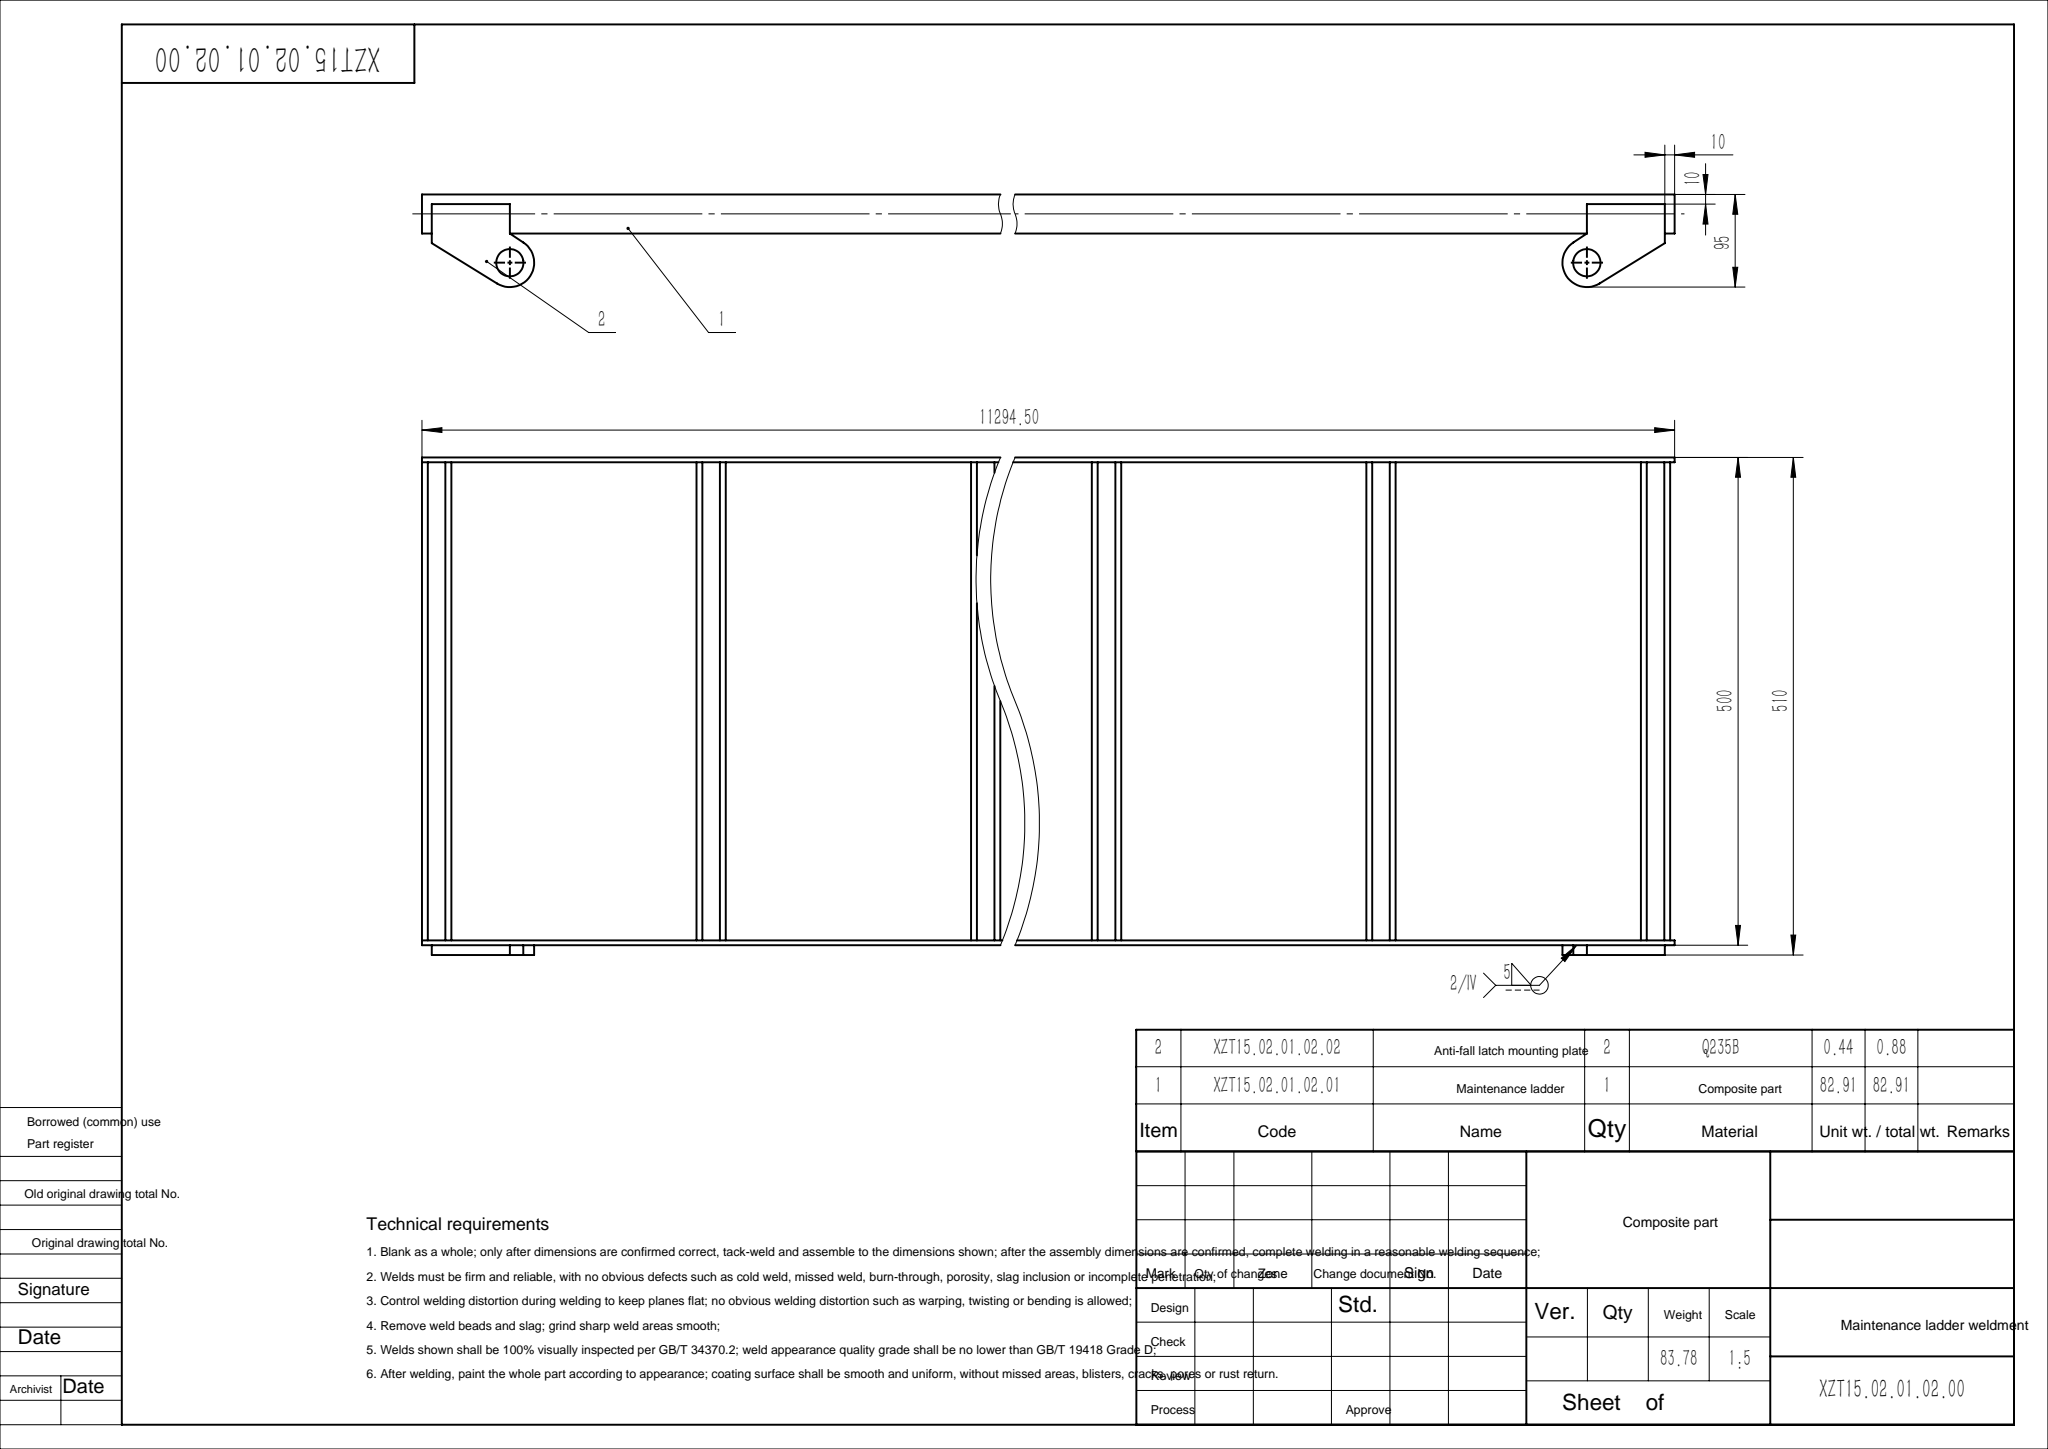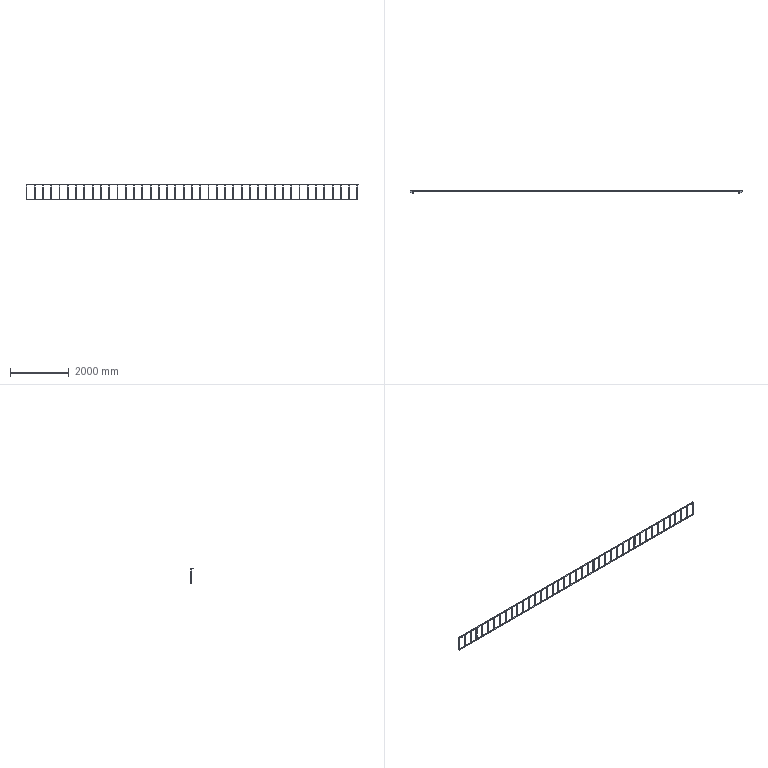Part | SolidWorks | features MirrorCompFeat 1, ReferencePattern 1 | 45 solids | 770 faces | box 11295 x 95 x 510 mm | volume 10672241 mm3 | plane 436 | cylinder 334 | commonest cylinder face diameters 6 x164 12 x164 28 x4 50 x2